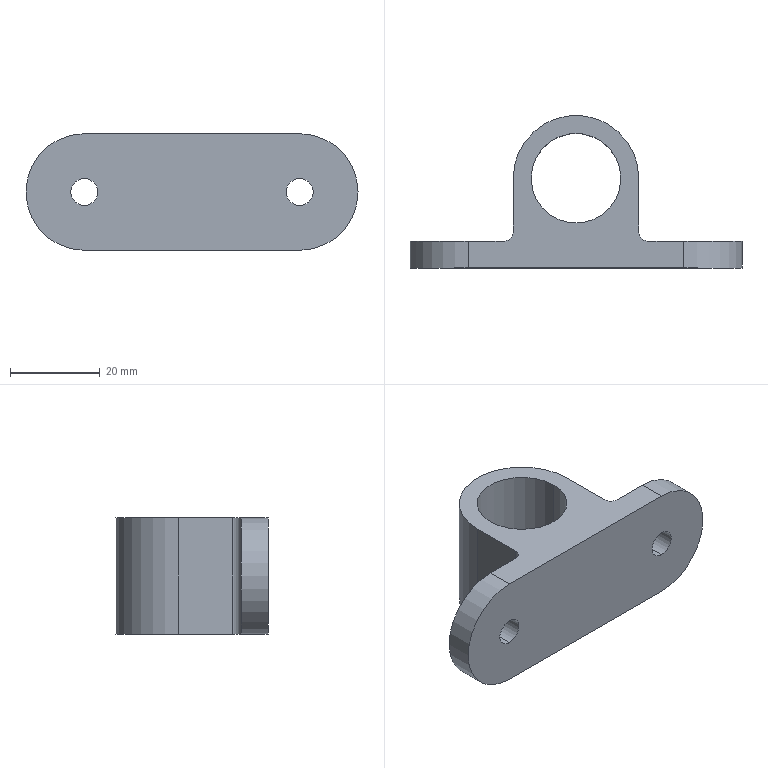Part | SolidWorks | features Extrusion 1, Fillet 1, ICE 1 | 1 solid | 18 faces | box 74 x 34 x 26 mm | volume 20408 mm3 | cylinder 11 | plane 7 | commonest cylinder face diameters 6 x4 4 x2 20 x2 26 x2 28 x1
STEP:
#1=CARTESIAN_POINT('',(-10.,20.,13.));
#2=VERTEX_POINT('',#1);
#3=CARTESIAN_POINT('',(10.,20.,13.));
#4=VERTEX_POINT('',#3);
#5=CARTESIAN_POINT('',(0.,20.,13.));
#6=DIRECTION('',(0.,0.,1.));
#7=DIRECTION('',(1.,0.,0.));
#8=AXIS2_PLACEMENT_3D('',#5,#6,#7);
#9=CIRCLE('',#8,10.);
#10=EDGE_CURVE('',#2,#4,#9,.T.);
#11=ORIENTED_EDGE('',*,*,#10,.T.);
#12=CARTESIAN_POINT('',(10.,20.,-13.));
#13=VERTEX_POINT('',#12);
#14=CARTESIAN_POINT('',(10.,20.,13.));
#15=DIRECTION('',(0.,0.,-1.));
#16=VECTOR('',#15,1000.);
#17=LINE('',#14,#16);
#18=EDGE_CURVE('',#4,#13,#17,.T.);
#19=ORIENTED_EDGE('',*,*,#18,.T.);
#20=CARTESIAN_POINT('',(-10.,20.,-13.));
#21=VERTEX_POINT('',#20);
#22=CARTESIAN_POINT('',(0.,20.,-13.));
#23=DIRECTION('',(0.,0.,1.));
#24=DIRECTION('',(1.,0.,0.));
#25=AXIS2_PLACEMENT_3D('',#22,#23,#24);
#26=CIRCLE('',#25,10.);
#27=EDGE_CURVE('',#21,#13,#26,.T.);
#28=ORIENTED_EDGE('',*,*,#27,.F.);
#29=CARTESIAN_POINT('',(-10.,20.,13.));
#30=DIRECTION('',(0.,0.,-1.));
#31=VECTOR('',#30,1000.);
#32=LINE('',#29,#31);
#33=EDGE_CURVE('',#2,#21,#32,.T.);
#34=ORIENTED_EDGE('',*,*,#33,.F.);
#35=EDGE_LOOP('',(#11,#19,#28,#34));
#36=FACE_OUTER_BOUND('',#35,.T.);
#37=CARTESIAN_POINT('',(0.,20.,13.));
#38=DIRECTION('',(0.,0.,-1.));
#39=DIRECTION('',(-1.,0.,0.));
#40=AXIS2_PLACEMENT_3D('',#37,#38,#39);
#41=CYLINDRICAL_SURFACE('',#40,10.);
#42=ADVANCED_FACE('',(#36),#41,.F.);
#43=CARTESIAN_POINT('',(24.,6.,-3.));
#44=VERTEX_POINT('',#43);
#45=CARTESIAN_POINT('',(24.,6.,3.));
#46=VERTEX_POINT('',#45);
#47=CARTESIAN_POINT('',(24.,6.,0.));
#48=DIRECTION('',(0.,1.,0.));
#49=DIRECTION('',(0.,0.,1.));
#50=AXIS2_PLACEMENT_3D('',#47,#48,#49);
#51=CIRCLE('',#50,3.);
#52=EDGE_CURVE('',#44,#46,#51,.T.);
#53=ORIENTED_EDGE('',*,*,#52,.T.);
#54=CARTESIAN_POINT('',(24.,0.,3.));
#55=VERTEX_POINT('',#54);
#56=CARTESIAN_POINT('',(24.,6.,3.));
#57=DIRECTION('',(0.,-1.,0.));
#58=VECTOR('',#57,1000.);
#59=LINE('',#56,#58);
#60=EDGE_CURVE('',#46,#55,#59,.T.);
#61=ORIENTED_EDGE('',*,*,#60,.T.);
#62=CARTESIAN_POINT('',(24.,0.,-3.));
#63=VERTEX_POINT('',#62);
#64=CARTESIAN_POINT('',(24.,0.,0.));
#65=DIRECTION('',(0.,1.,0.));
#66=DIRECTION('',(0.,0.,1.));
#67=AXIS2_PLACEMENT_3D('',#64,#65,#66);
#68=CIRCLE('',#67,3.);
#69=EDGE_CURVE('',#63,#55,#68,.T.);
#70=ORIENTED_EDGE('',*,*,#69,.F.);
#71=CARTESIAN_POINT('',(24.,6.,-3.));
#72=DIRECTION('',(0.,-1.,0.));
#73=VECTOR('',#72,1000.);
#74=LINE('',#71,#73);
#75=EDGE_CURVE('',#44,#63,#74,.T.);
#76=ORIENTED_EDGE('',*,*,#75,.F.);
#77=EDGE_LOOP('',(#53,#61,#70,#76));
#78=FACE_OUTER_BOUND('',#77,.T.);
#79=CARTESIAN_POINT('',(24.,6.,0.));
#80=DIRECTION('',(0.,-1.,0.));
#81=DIRECTION('',(0.,0.,-1.));
#82=AXIS2_PLACEMENT_3D('',#79,#80,#81);
#83=CYLINDRICAL_SURFACE('',#82,3.);
#84=ADVANCED_FACE('',(#78),#83,.F.);
#85=CARTESIAN_POINT('',(-24.,6.,-3.));
#86=VERTEX_POINT('',#85);
#87=CARTESIAN_POINT('',(-24.,6.,3.));
#88=VERTEX_POINT('',#87);
#89=CARTESIAN_POINT('',(-24.,6.,0.));
#90=DIRECTION('',(0.,1.,0.));
#91=DIRECTION('',(0.,0.,1.));
#92=AXIS2_PLACEMENT_3D('',#89,#90,#91);
#93=CIRCLE('',#92,3.);
#94=EDGE_CURVE('',#86,#88,#93,.T.);
#95=ORIENTED_EDGE('',*,*,#94,.T.);
#96=CARTESIAN_POINT('',(-24.,0.,3.));
#97=VERTEX_POINT('',#96);
#98=CARTESIAN_POINT('',(-24.,6.,3.));
#99=DIRECTION('',(0.,-1.,0.));
#100=VECTOR('',#99,1000.);
#101=LINE('',#98,#100);
#102=EDGE_CURVE('',#88,#97,#101,.T.);
#103=ORIENTED_EDGE('',*,*,#102,.T.);
#104=CARTESIAN_POINT('',(-24.,0.,-3.));
#105=VERTEX_POINT('',#104);
#106=CARTESIAN_POINT('',(-24.,0.,0.));
#107=DIRECTION('',(0.,1.,0.));
#108=DIRECTION('',(0.,0.,1.));
#109=AXIS2_PLACEMENT_3D('',#106,#107,#108);
#110=CIRCLE('',#109,3.);
#111=EDGE_CURVE('',#105,#97,#110,.T.);
#112=ORIENTED_EDGE('',*,*,#111,.F.);
#113=CARTESIAN_POINT('',(-24.,6.,-3.));
#114=DIRECTION('',(0.,-1.,0.));
#115=VECTOR('',#114,1000.);
#116=LINE('',#113,#115);
#117=EDGE_CURVE('',#86,#105,#116,.T.);
#118=ORIENTED_EDGE('',*,*,#117,.F.);
#119=EDGE_LOOP('',(#95,#103,#112,#118));
#120=FACE_OUTER_BOUND('',#119,.T.);
#121=CARTESIAN_POINT('',(-24.,6.,0.));
#122=DIRECTION('',(0.,-1.,0.));
#123=DIRECTION('',(0.,0.,-1.));
#124=AXIS2_PLACEMENT_3D('',#121,#122,#123);
#125=CYLINDRICAL_SURFACE('',#124,3.);
#126=ADVANCED_FACE('',(#120),#125,.F.);
#127=ORIENTED_EDGE('',*,*,#94,.F.);
#128=CARTESIAN_POINT('',(-24.,6.,0.));
#129=DIRECTION('',(0.,1.,0.));
#130=DIRECTION('',(0.,0.,1.));
#131=AXIS2_PLACEMENT_3D('',#128,#129,#130);
#132=CIRCLE('',#131,3.);
#133=EDGE_CURVE('',#88,#86,#132,.T.);
#134=ORIENTED_EDGE('',*,*,#133,.F.);
#135=EDGE_LOOP('',(#127,#134));
#136=FACE_BOUND('',#135,.T.);
#137=CARTESIAN_POINT('',(-24.,6.,13.));
#138=VERTEX_POINT('',#137);
#139=CARTESIAN_POINT('',(-16.,6.,13.));
#140=VERTEX_POINT('',#139);
#141=CARTESIAN_POINT('',(-24.,6.,13.));
#142=DIRECTION('',(1.,0.,0.));
#143=VECTOR('',#142,1000.);
#144=LINE('',#141,#143);
#145=EDGE_CURVE('',#138,#140,#144,.T.);
#146=ORIENTED_EDGE('',*,*,#145,.T.);
#147=CARTESIAN_POINT('',(-16.,6.,-13.));
#148=VERTEX_POINT('',#147);
#149=CARTESIAN_POINT('',(-16.,6.,0.));
#150=DIRECTION('',(0.,0.,-1.));
#151=VECTOR('',#150,1000.);
#152=LINE('',#149,#151);
#153=EDGE_CURVE('',#140,#148,#152,.T.);
#154=ORIENTED_EDGE('',*,*,#153,.T.);
#155=CARTESIAN_POINT('',(-24.,6.,-13.));
#156=VERTEX_POINT('',#155);
#157=CARTESIAN_POINT('',(-24.,6.,-13.));
#158=DIRECTION('',(-1.,0.,0.));
#159=VECTOR('',#158,1000.);
#160=LINE('',#157,#159);
#161=EDGE_CURVE('',#148,#156,#160,.T.);
#162=ORIENTED_EDGE('',*,*,#161,.T.);
#163=CARTESIAN_POINT('',(-24.,6.,0.));
#164=DIRECTION('',(0.,1.,0.));
#165=DIRECTION('',(0.,0.,1.));
#166=AXIS2_PLACEMENT_3D('',#163,#164,#165);
#167=CIRCLE('',#166,13.);
#168=EDGE_CURVE('',#156,#138,#167,.T.);
#169=ORIENTED_EDGE('',*,*,#168,.T.);
#170=EDGE_LOOP('',(#146,#154,#162,#169));
#171=FACE_OUTER_BOUND('',#170,.T.);
#172=CARTESIAN_POINT('',(-24.,6.,0.));
#173=DIRECTION('',(0.,1.,0.));
#174=DIRECTION('',(0.,0.,1.));
#175=AXIS2_PLACEMENT_3D('',#172,#173,#174);
#176=PLANE('',#175);
#177=ADVANCED_FACE('',(#136,#171),#176,.T.);
#178=ORIENTED_EDGE('',*,*,#52,.F.);
#179=CARTESIAN_POINT('',(24.,6.,0.));
#180=DIRECTION('',(0.,1.,0.));
#181=DIRECTION('',(0.,0.,1.));
#182=AXIS2_PLACEMENT_3D('',#179,#180,#181);
#183=CIRCLE('',#182,3.);
#184=EDGE_CURVE('',#46,#44,#183,.T.);
#185=ORIENTED_EDGE('',*,*,#184,.F.);
#186=EDGE_LOOP('',(#178,#185));
#187=FACE_BOUND('',#186,.T.);
#188=CARTESIAN_POINT('',(24.,6.,-13.));
#189=VERTEX_POINT('',#188);
#190=CARTESIAN_POINT('',(16.,6.,-13.));
#191=VERTEX_POINT('',#190);
#192=CARTESIAN_POINT('',(-24.,6.,-13.));
#193=DIRECTION('',(-1.,0.,0.));
#194=VECTOR('',#193,1000.);
#195=LINE('',#192,#194);
#196=EDGE_CURVE('',#189,#191,#195,.T.);
#197=ORIENTED_EDGE('',*,*,#196,.T.);
#198=CARTESIAN_POINT('',(16.,6.,13.));
#199=VERTEX_POINT('',#198);
#200=CARTESIAN_POINT('',(16.,6.,0.));
#201=DIRECTION('',(0.,0.,1.));
#202=VECTOR('',#201,1000.);
#203=LINE('',#200,#202);
#204=EDGE_CURVE('',#191,#199,#203,.T.);
#205=ORIENTED_EDGE('',*,*,#204,.T.);
#206=CARTESIAN_POINT('',(24.,6.,13.));
#207=VERTEX_POINT('',#206);
#208=CARTESIAN_POINT('',(-24.,6.,13.));
#209=DIRECTION('',(1.,0.,0.));
#210=VECTOR('',#209,1000.);
#211=LINE('',#208,#210);
#212=EDGE_CURVE('',#199,#207,#211,.T.);
#213=ORIENTED_EDGE('',*,*,#212,.T.);
#214=CARTESIAN_POINT('',(24.,6.,0.));
#215=DIRECTION('',(0.,1.,0.));
#216=DIRECTION('',(0.,0.,1.));
#217=AXIS2_PLACEMENT_3D('',#214,#215,#216);
#218=CIRCLE('',#217,13.);
#219=EDGE_CURVE('',#207,#189,#218,.T.);
#220=ORIENTED_EDGE('',*,*,#219,.T.);
#221=EDGE_LOOP('',(#197,#205,#213,#220));
#222=FACE_OUTER_BOUND('',#221,.T.);
#223=CARTESIAN_POINT('',(-24.,6.,0.));
#224=DIRECTION('',(0.,1.,0.));
#225=DIRECTION('',(0.,0.,1.));
#226=AXIS2_PLACEMENT_3D('',#223,#224,#225);
#227=PLANE('',#226);
#228=ADVANCED_FACE('',(#187,#222),#227,.T.);
#229=CARTESIAN_POINT('',(24.,0.,13.));
#230=VERTEX_POINT('',#229);
#231=CARTESIAN_POINT('',(24.,0.,-13.));
#232=VERTEX_POINT('',#231);
#233=CARTESIAN_POINT('',(24.,0.,0.));
#234=DIRECTION('',(0.,1.,0.));
#235=DIRECTION('',(0.,0.,1.));
#236=AXIS2_PLACEMENT_3D('',#233,#234,#235);
#237=CIRCLE('',#236,13.);
#238=EDGE_CURVE('',#230,#232,#237,.T.);
#239=ORIENTED_EDGE('',*,*,#238,.F.);
#240=CARTESIAN_POINT('',(-24.,0.,13.));
#241=VERTEX_POINT('',#240);
#242=CARTESIAN_POINT('',(-24.,0.,13.));
#243=DIRECTION('',(1.,0.,0.));
#244=VECTOR('',#243,1000.);
#245=LINE('',#242,#244);
#246=EDGE_CURVE('',#241,#230,#245,.T.);
#247=ORIENTED_EDGE('',*,*,#246,.F.);
#248=CARTESIAN_POINT('',(-24.,0.,-13.));
#249=VERTEX_POINT('',#248);
#250=CARTESIAN_POINT('',(-24.,0.,0.));
#251=DIRECTION('',(0.,1.,0.));
#252=DIRECTION('',(0.,0.,1.));
#253=AXIS2_PLACEMENT_3D('',#250,#251,#252);
#254=CIRCLE('',#253,13.);
#255=EDGE_CURVE('',#249,#241,#254,.T.);
#256=ORIENTED_EDGE('',*,*,#255,.F.);
#257=CARTESIAN_POINT('',(-24.,0.,-13.));
#258=DIRECTION('',(-1.,0.,0.));
#259=VECTOR('',#258,1000.);
#260=LINE('',#257,#259);
#261=EDGE_CURVE('',#232,#249,#260,.T.);
#262=ORIENTED_EDGE('',*,*,#261,.F.);
#263=EDGE_LOOP('',(#239,#247,#256,#262));
#264=FACE_OUTER_BOUND('',#263,.T.);
#265=ORIENTED_EDGE('',*,*,#69,.T.);
#266=CARTESIAN_POINT('',(24.,0.,0.));
#267=DIRECTION('',(0.,1.,0.));
#268=DIRECTION('',(0.,0.,1.));
#269=AXIS2_PLACEMENT_3D('',#266,#267,#268);
#270=CIRCLE('',#269,3.);
#271=EDGE_CURVE('',#55,#63,#270,.T.);
#272=ORIENTED_EDGE('',*,*,#271,.T.);
#273=EDGE_LOOP('',(#265,#272));
#274=FACE_BOUND('',#273,.T.);
#275=ORIENTED_EDGE('',*,*,#111,.T.);
#276=CARTESIAN_POINT('',(-24.,0.,0.));
#277=DIRECTION('',(0.,1.,0.));
#278=DIRECTION('',(0.,0.,1.));
#279=AXIS2_PLACEMENT_3D('',#276,#277,#278);
#280=CIRCLE('',#279,3.);
#281=EDGE_CURVE('',#97,#105,#280,.T.);
#282=ORIENTED_EDGE('',*,*,#281,.T.);
#283=EDGE_LOOP('',(#275,#282));
#284=FACE_BOUND('',#283,.T.);
#285=CARTESIAN_POINT('',(-24.,0.,0.));
#286=DIRECTION('',(0.,1.,0.));
#287=DIRECTION('',(0.,0.,1.));
#288=AXIS2_PLACEMENT_3D('',#285,#286,#287);
#289=PLANE('',#288);
#290=ADVANCED_FACE('',(#264,#274,#284),#289,.F.);
#291=ORIENTED_EDGE('',*,*,#255,.T.);
#292=CARTESIAN_POINT('',(-24.,6.,13.));
#293=DIRECTION('',(0.,-1.,0.));
#294=VECTOR('',#293,1000.);
#295=LINE('',#292,#294);
#296=EDGE_CURVE('',#138,#241,#295,.T.);
#297=ORIENTED_EDGE('',*,*,#296,.F.);
#298=ORIENTED_EDGE('',*,*,#168,.F.);
#299=CARTESIAN_POINT('',(-24.,6.,-13.));
#300=DIRECTION('',(0.,-1.,0.));
#301=VECTOR('',#300,1000.);
#302=LINE('',#299,#301);
#303=EDGE_CURVE('',#156,#249,#302,.T.);
#304=ORIENTED_EDGE('',*,*,#303,.T.);
#305=EDGE_LOOP('',(#291,#297,#298,#304));
#306=FACE_OUTER_BOUND('',#305,.T.);
#307=CARTESIAN_POINT('',(-24.,6.,0.));
#308=DIRECTION('',(0.,-1.,0.));
#309=DIRECTION('',(0.,0.,-1.));
#310=AXIS2_PLACEMENT_3D('',#307,#308,#309);
#311=CYLINDRICAL_SURFACE('',#310,13.);
#312=ADVANCED_FACE('',(#306),#311,.T.);
#313=ORIENTED_EDGE('',*,*,#212,.F.);
#314=CARTESIAN_POINT('',(14.,8.,13.));
#315=VERTEX_POINT('',#314);
#316=CARTESIAN_POINT('',(16.,8.,13.));
#317=DIRECTION('',(0.,0.,-1.));
#318=DIRECTION('',(-1.,0.,0.));
#319=AXIS2_PLACEMENT_3D('',#316,#317,#318);
#320=CIRCLE('',#319,2.);
#321=EDGE_CURVE('',#199,#315,#320,.T.);
#322=ORIENTED_EDGE('',*,*,#321,.T.);
#323=CARTESIAN_POINT('',(14.,20.,13.));
#324=VERTEX_POINT('',#323);
#325=CARTESIAN_POINT('',(14.,20.,13.));
#326=DIRECTION('',(0.,1.,0.));
#327=VECTOR('',#326,1000.);
#328=LINE('',#325,#327);
#329=EDGE_CURVE('',#315,#324,#328,.T.);
#330=ORIENTED_EDGE('',*,*,#329,.T.);
#331=CARTESIAN_POINT('',(-14.,20.,13.));
#332=VERTEX_POINT('',#331);
#333=CARTESIAN_POINT('',(0.,20.,13.));
#334=DIRECTION('',(0.,0.,1.));
#335=DIRECTION('',(1.,0.,0.));
#336=AXIS2_PLACEMENT_3D('',#333,#334,#335);
#337=CIRCLE('',#336,14.);
#338=EDGE_CURVE('',#324,#332,#337,.T.);
#339=ORIENTED_EDGE('',*,*,#338,.T.);
#340=CARTESIAN_POINT('',(-14.,8.,13.));
#341=VERTEX_POINT('',#340);
#342=CARTESIAN_POINT('',(-14.,20.,13.));
#343=DIRECTION('',(0.,-1.,0.));
#344=VECTOR('',#343,1000.);
#345=LINE('',#342,#344);
#346=EDGE_CURVE('',#332,#341,#345,.T.);
#347=ORIENTED_EDGE('',*,*,#346,.T.);
#348=CARTESIAN_POINT('',(-16.,8.,13.));
#349=DIRECTION('',(0.,0.,-1.));
#350=DIRECTION('',(-1.,0.,0.));
#351=AXIS2_PLACEMENT_3D('',#348,#349,#350);
#352=CIRCLE('',#351,2.);
#353=EDGE_CURVE('',#341,#140,#352,.T.);
#354=ORIENTED_EDGE('',*,*,#353,.T.);
#355=ORIENTED_EDGE('',*,*,#145,.F.);
#356=ORIENTED_EDGE('',*,*,#296,.T.);
#357=ORIENTED_EDGE('',*,*,#246,.T.);
#358=CARTESIAN_POINT('',(24.,6.,13.));
#359=DIRECTION('',(0.,-1.,0.));
#360=VECTOR('',#359,1000.);
#361=LINE('',#358,#360);
#362=EDGE_CURVE('',#207,#230,#361,.T.);
#363=ORIENTED_EDGE('',*,*,#362,.F.);
#364=EDGE_LOOP('',(#313,#322,#330,#339,#347,#354,#355,#356,#357,#363));
#365=FACE_OUTER_BOUND('',#364,.T.);
#366=ORIENTED_EDGE('',*,*,#10,.F.);
#367=CARTESIAN_POINT('',(0.,20.,13.));
#368=DIRECTION('',(0.,0.,1.));
#369=DIRECTION('',(1.,0.,0.));
#370=AXIS2_PLACEMENT_3D('',#367,#368,#369);
#371=CIRCLE('',#370,10.);
#372=EDGE_CURVE('',#4,#2,#371,.T.);
#373=ORIENTED_EDGE('',*,*,#372,.F.);
#374=EDGE_LOOP('',(#366,#373));
#375=FACE_BOUND('',#374,.T.);
#376=CARTESIAN_POINT('',(-24.,6.,13.));
#377=DIRECTION('',(0.,0.,-1.));
#378=DIRECTION('',(-1.,0.,0.));
#379=AXIS2_PLACEMENT_3D('',#376,#377,#378);
#380=PLANE('',#379);
#381=ADVANCED_FACE('',(#365,#375),#380,.F.);
#382=ORIENTED_EDGE('',*,*,#238,.T.);
#383=CARTESIAN_POINT('',(24.,6.,-13.));
#384=DIRECTION('',(0.,-1.,0.));
#385=VECTOR('',#384,1000.);
#386=LINE('',#383,#385);
#387=EDGE_CURVE('',#189,#232,#386,.T.);
#388=ORIENTED_EDGE('',*,*,#387,.F.);
#389=ORIENTED_EDGE('',*,*,#219,.F.);
#390=ORIENTED_EDGE('',*,*,#362,.T.);
#391=EDGE_LOOP('',(#382,#388,#389,#390));
#392=FACE_OUTER_BOUND('',#391,.T.);
#393=CARTESIAN_POINT('',(24.,6.,0.));
#394=DIRECTION('',(0.,-1.,0.));
#395=DIRECTION('',(0.,0.,-1.));
#396=AXIS2_PLACEMENT_3D('',#393,#394,#395);
#397=CYLINDRICAL_SURFACE('',#396,13.);
#398=ADVANCED_FACE('',(#392),#397,.T.);
#399=ORIENTED_EDGE('',*,*,#261,.T.);
#400=ORIENTED_EDGE('',*,*,#303,.F.);
#401=ORIENTED_EDGE('',*,*,#161,.F.);
#402=CARTESIAN_POINT('',(-14.,8.,-13.));
#403=VERTEX_POINT('',#402);
#404=CARTESIAN_POINT('',(-16.,8.,-13.));
#405=DIRECTION('',(0.,0.,1.));
#406=DIRECTION('',(1.,0.,0.));
#407=AXIS2_PLACEMENT_3D('',#404,#405,#406);
#408=CIRCLE('',#407,2.);
#409=EDGE_CURVE('',#148,#403,#408,.T.);
#410=ORIENTED_EDGE('',*,*,#409,.T.);
#411=CARTESIAN_POINT('',(-14.,20.,-13.));
#412=VERTEX_POINT('',#411);
#413=CARTESIAN_POINT('',(-14.,20.,-13.));
#414=DIRECTION('',(0.,-1.,0.));
#415=VECTOR('',#414,1000.);
#416=LINE('',#413,#415);
#417=EDGE_CURVE('',#412,#403,#416,.T.);
#418=ORIENTED_EDGE('',*,*,#417,.F.);
#419=CARTESIAN_POINT('',(14.,20.,-13.));
#420=VERTEX_POINT('',#419);
#421=CARTESIAN_POINT('',(0.,20.,-13.));
#422=DIRECTION('',(0.,0.,1.));
#423=DIRECTION('',(1.,0.,0.));
#424=AXIS2_PLACEMENT_3D('',#421,#422,#423);
#425=CIRCLE('',#424,14.);
#426=EDGE_CURVE('',#420,#412,#425,.T.);
#427=ORIENTED_EDGE('',*,*,#426,.F.);
#428=CARTESIAN_POINT('',(14.,8.,-13.));
#429=VERTEX_POINT('',#428);
#430=CARTESIAN_POINT('',(14.,20.,-13.));
#431=DIRECTION('',(0.,1.,0.));
#432=VECTOR('',#431,1000.);
#433=LINE('',#430,#432);
#434=EDGE_CURVE('',#429,#420,#433,.T.);
#435=ORIENTED_EDGE('',*,*,#434,.F.);
#436=CARTESIAN_POINT('',(16.,8.,-13.));
#437=DIRECTION('',(0.,0.,1.));
#438=DIRECTION('',(1.,0.,0.));
#439=AXIS2_PLACEMENT_3D('',#436,#437,#438);
#440=CIRCLE('',#439,2.);
#441=EDGE_CURVE('',#429,#191,#440,.T.);
#442=ORIENTED_EDGE('',*,*,#441,.T.);
#443=ORIENTED_EDGE('',*,*,#196,.F.);
#444=ORIENTED_EDGE('',*,*,#387,.T.);
#445=EDGE_LOOP('',(#399,#400,#401,#410,#418,#427,#435,#442,#443,#444));
#446=FACE_OUTER_BOUND('',#445,.T.);
#447=ORIENTED_EDGE('',*,*,#27,.T.);
#448=CARTESIAN_POINT('',(0.,20.,-13.));
#449=DIRECTION('',(0.,0.,1.));
#450=DIRECTION('',(1.,0.,0.));
#451=AXIS2_PLACEMENT_3D('',#448,#449,#450);
#452=CIRCLE('',#451,10.);
#453=EDGE_CURVE('',#13,#21,#452,.T.);
#454=ORIENTED_EDGE('',*,*,#453,.T.);
#455=EDGE_LOOP('',(#447,#454));
#456=FACE_BOUND('',#455,.T.);
#457=CARTESIAN_POINT('',(-24.,6.,-13.));
#458=DIRECTION('',(0.,0.,1.));
#459=DIRECTION('',(1.,0.,0.));
#460=AXIS2_PLACEMENT_3D('',#457,#458,#459);
#461=PLANE('',#460);
#462=ADVANCED_FACE('',(#446,#456),#461,.F.);
#463=ORIENTED_EDGE('',*,*,#102,.F.);
#464=ORIENTED_EDGE('',*,*,#133,.T.);
#465=ORIENTED_EDGE('',*,*,#117,.T.);
#466=ORIENTED_EDGE('',*,*,#281,.F.);
#467=EDGE_LOOP('',(#463,#464,#465,#466));
#468=FACE_OUTER_BOUND('',#467,.T.);
#469=CARTESIAN_POINT('',(-24.,6.,0.));
#470=DIRECTION('',(0.,-1.,0.));
#471=DIRECTION('',(0.,0.,-1.));
#472=AXIS2_PLACEMENT_3D('',#469,#470,#471);
#473=CYLINDRICAL_SURFACE('',#472,3.);
#474=ADVANCED_FACE('',(#468),#473,.F.);
#475=ORIENTED_EDGE('',*,*,#60,.F.);
#476=ORIENTED_EDGE('',*,*,#184,.T.);
#477=ORIENTED_EDGE('',*,*,#75,.T.);
#478=ORIENTED_EDGE('',*,*,#271,.F.);
#479=EDGE_LOOP('',(#475,#476,#477,#478));
#480=FACE_OUTER_BOUND('',#479,.T.);
#481=CARTESIAN_POINT('',(24.,6.,0.));
#482=DIRECTION('',(0.,-1.,0.));
#483=DIRECTION('',(0.,0.,-1.));
#484=AXIS2_PLACEMENT_3D('',#481,#482,#483);
#485=CYLINDRICAL_SURFACE('',#484,3.);
#486=ADVANCED_FACE('',(#480),#485,.F.);
#487=ORIENTED_EDGE('',*,*,#426,.T.);
#488=CARTESIAN_POINT('',(-14.,20.,13.));
#489=DIRECTION('',(0.,0.,-1.));
#490=VECTOR('',#489,1000.);
#491=LINE('',#488,#490);
#492=EDGE_CURVE('',#332,#412,#491,.T.);
#493=ORIENTED_EDGE('',*,*,#492,.F.);
#494=ORIENTED_EDGE('',*,*,#338,.F.);
#495=CARTESIAN_POINT('',(14.,20.,13.));
#496=DIRECTION('',(0.,0.,-1.));
#497=VECTOR('',#496,1000.);
#498=LINE('',#495,#497);
#499=EDGE_CURVE('',#324,#420,#498,.T.);
#500=ORIENTED_EDGE('',*,*,#499,.T.);
#501=EDGE_LOOP('',(#487,#493,#494,#500));
#502=FACE_OUTER_BOUND('',#501,.T.);
#503=CARTESIAN_POINT('',(0.,20.,13.));
#504=DIRECTION('',(0.,0.,-1.));
#505=DIRECTION('',(-1.,0.,0.));
#506=AXIS2_PLACEMENT_3D('',#503,#504,#505);
#507=CYLINDRICAL_SURFACE('',#506,14.);
#508=ADVANCED_FACE('',(#502),#507,.T.);
#509=ORIENTED_EDGE('',*,*,#417,.T.);
#510=CARTESIAN_POINT('',(-14.,8.,13.));
#511=DIRECTION('',(0.,0.,1.));
#512=VECTOR('',#511,1000.);
#513=LINE('',#510,#512);
#514=EDGE_CURVE('',#403,#341,#513,.T.);
#515=ORIENTED_EDGE('',*,*,#514,.T.);
#516=ORIENTED_EDGE('',*,*,#346,.F.);
#517=ORIENTED_EDGE('',*,*,#492,.T.);
#518=EDGE_LOOP('',(#509,#515,#516,#517));
#519=FACE_OUTER_BOUND('',#518,.T.);
#520=CARTESIAN_POINT('',(-14.,20.,13.));
#521=DIRECTION('',(1.,0.,0.));
#522=DIRECTION('',(0.,0.,-1.));
#523=AXIS2_PLACEMENT_3D('',#520,#521,#522);
#524=PLANE('',#523);
#525=ADVANCED_FACE('',(#519),#524,.F.);
#526=ORIENTED_EDGE('',*,*,#329,.F.);
#527=CARTESIAN_POINT('',(14.,8.,13.));
#528=DIRECTION('',(0.,0.,-1.));
#529=VECTOR('',#528,1000.);
#530=LINE('',#527,#529);
#531=EDGE_CURVE('',#315,#429,#530,.T.);
#532=ORIENTED_EDGE('',*,*,#531,.T.);
#533=ORIENTED_EDGE('',*,*,#434,.T.);
#534=ORIENTED_EDGE('',*,*,#499,.F.);
#535=EDGE_LOOP('',(#526,#532,#533,#534));
#536=FACE_OUTER_BOUND('',#535,.T.);
#537=CARTESIAN_POINT('',(14.,20.,13.));
#538=DIRECTION('',(-1.,0.,0.));
#539=DIRECTION('',(0.,0.,1.));
#540=AXIS2_PLACEMENT_3D('',#537,#538,#539);
#541=PLANE('',#540);
#542=ADVANCED_FACE('',(#536),#541,.F.);
#543=ORIENTED_EDGE('',*,*,#18,.F.);
#544=ORIENTED_EDGE('',*,*,#372,.T.);
#545=ORIENTED_EDGE('',*,*,#33,.T.);
#546=ORIENTED_EDGE('',*,*,#453,.F.);
#547=EDGE_LOOP('',(#543,#544,#545,#546));
#548=FACE_OUTER_BOUND('',#547,.T.);
#549=CARTESIAN_POINT('',(0.,20.,13.));
#550=DIRECTION('',(0.,0.,-1.));
#551=DIRECTION('',(-1.,0.,0.));
#552=AXIS2_PLACEMENT_3D('',#549,#550,#551);
#553=CYLINDRICAL_SURFACE('',#552,10.);
#554=ADVANCED_FACE('',(#548),#553,.F.);
#555=ORIENTED_EDGE('',*,*,#441,.F.);
#556=ORIENTED_EDGE('',*,*,#531,.F.);
#557=ORIENTED_EDGE('',*,*,#321,.F.);
#558=ORIENTED_EDGE('',*,*,#204,.F.);
#559=EDGE_LOOP('',(#555,#556,#557,#558));
#560=FACE_OUTER_BOUND('',#559,.T.);
#561=CARTESIAN_POINT('',(16.,8.,0.));
#562=DIRECTION('',(0.,0.,1.));
#563=DIRECTION('',(1.,0.,0.));
#564=AXIS2_PLACEMENT_3D('',#561,#562,#563);
#565=CYLINDRICAL_SURFACE('',#564,2.);
#566=ADVANCED_FACE('',(#560),#565,.F.);
#567=ORIENTED_EDGE('',*,*,#353,.F.);
#568=ORIENTED_EDGE('',*,*,#514,.F.);
#569=ORIENTED_EDGE('',*,*,#409,.F.);
#570=ORIENTED_EDGE('',*,*,#153,.F.);
#571=EDGE_LOOP('',(#567,#568,#569,#570));
#572=FACE_OUTER_BOUND('',#571,.T.);
#573=CARTESIAN_POINT('',(-16.,8.,0.));
#574=DIRECTION('',(0.,0.,-1.));
#575=DIRECTION('',(-1.,0.,0.));
#576=AXIS2_PLACEMENT_3D('',#573,#574,#575);
#577=CYLINDRICAL_SURFACE('',#576,2.);
#578=ADVANCED_FACE('',(#572),#577,.F.);
#579=CLOSED_SHELL('',(#42,#84,#126,#177,#228,#290,#312,#381,#398,#462,#474,#486,#508,#525,#542,#554,#566,#578));
#580=MANIFOLD_SOLID_BREP('',#579);
#581=CARTESIAN_POINT('',(0.,0.,0.));
#582=DIRECTION('',(0.,0.,1.));
#583=DIRECTION('',(1.,0.,0.));
#584=AXIS2_PLACEMENT_3D('',#581,#582,#583);
#585=(LENGTH_UNIT()NAMED_UNIT(*)SI_UNIT(.MILLI.,.METRE.));
#586=UNCERTAINTY_MEASURE_WITH_UNIT(LENGTH_MEASURE(0.00001),#585,'','');
#587=(NAMED_UNIT(*)PLANE_ANGLE_UNIT()SI_UNIT($,.RADIAN.));
#588=(NAMED_UNIT(*)SI_UNIT($,.STERADIAN.)SOLID_ANGLE_UNIT());
#589=(GEOMETRIC_REPRESENTATION_CONTEXT(3)GLOBAL_UNCERTAINTY_ASSIGNED_CONTEXT((#586))GLOBAL_UNIT_ASSIGNED_CONTEXT((#585,#587,#588))REPRESENTATION_CONTEXT('',''));
#590=ADVANCED_BREP_SHAPE_REPRESENTATION('',(#580,#584),#589);